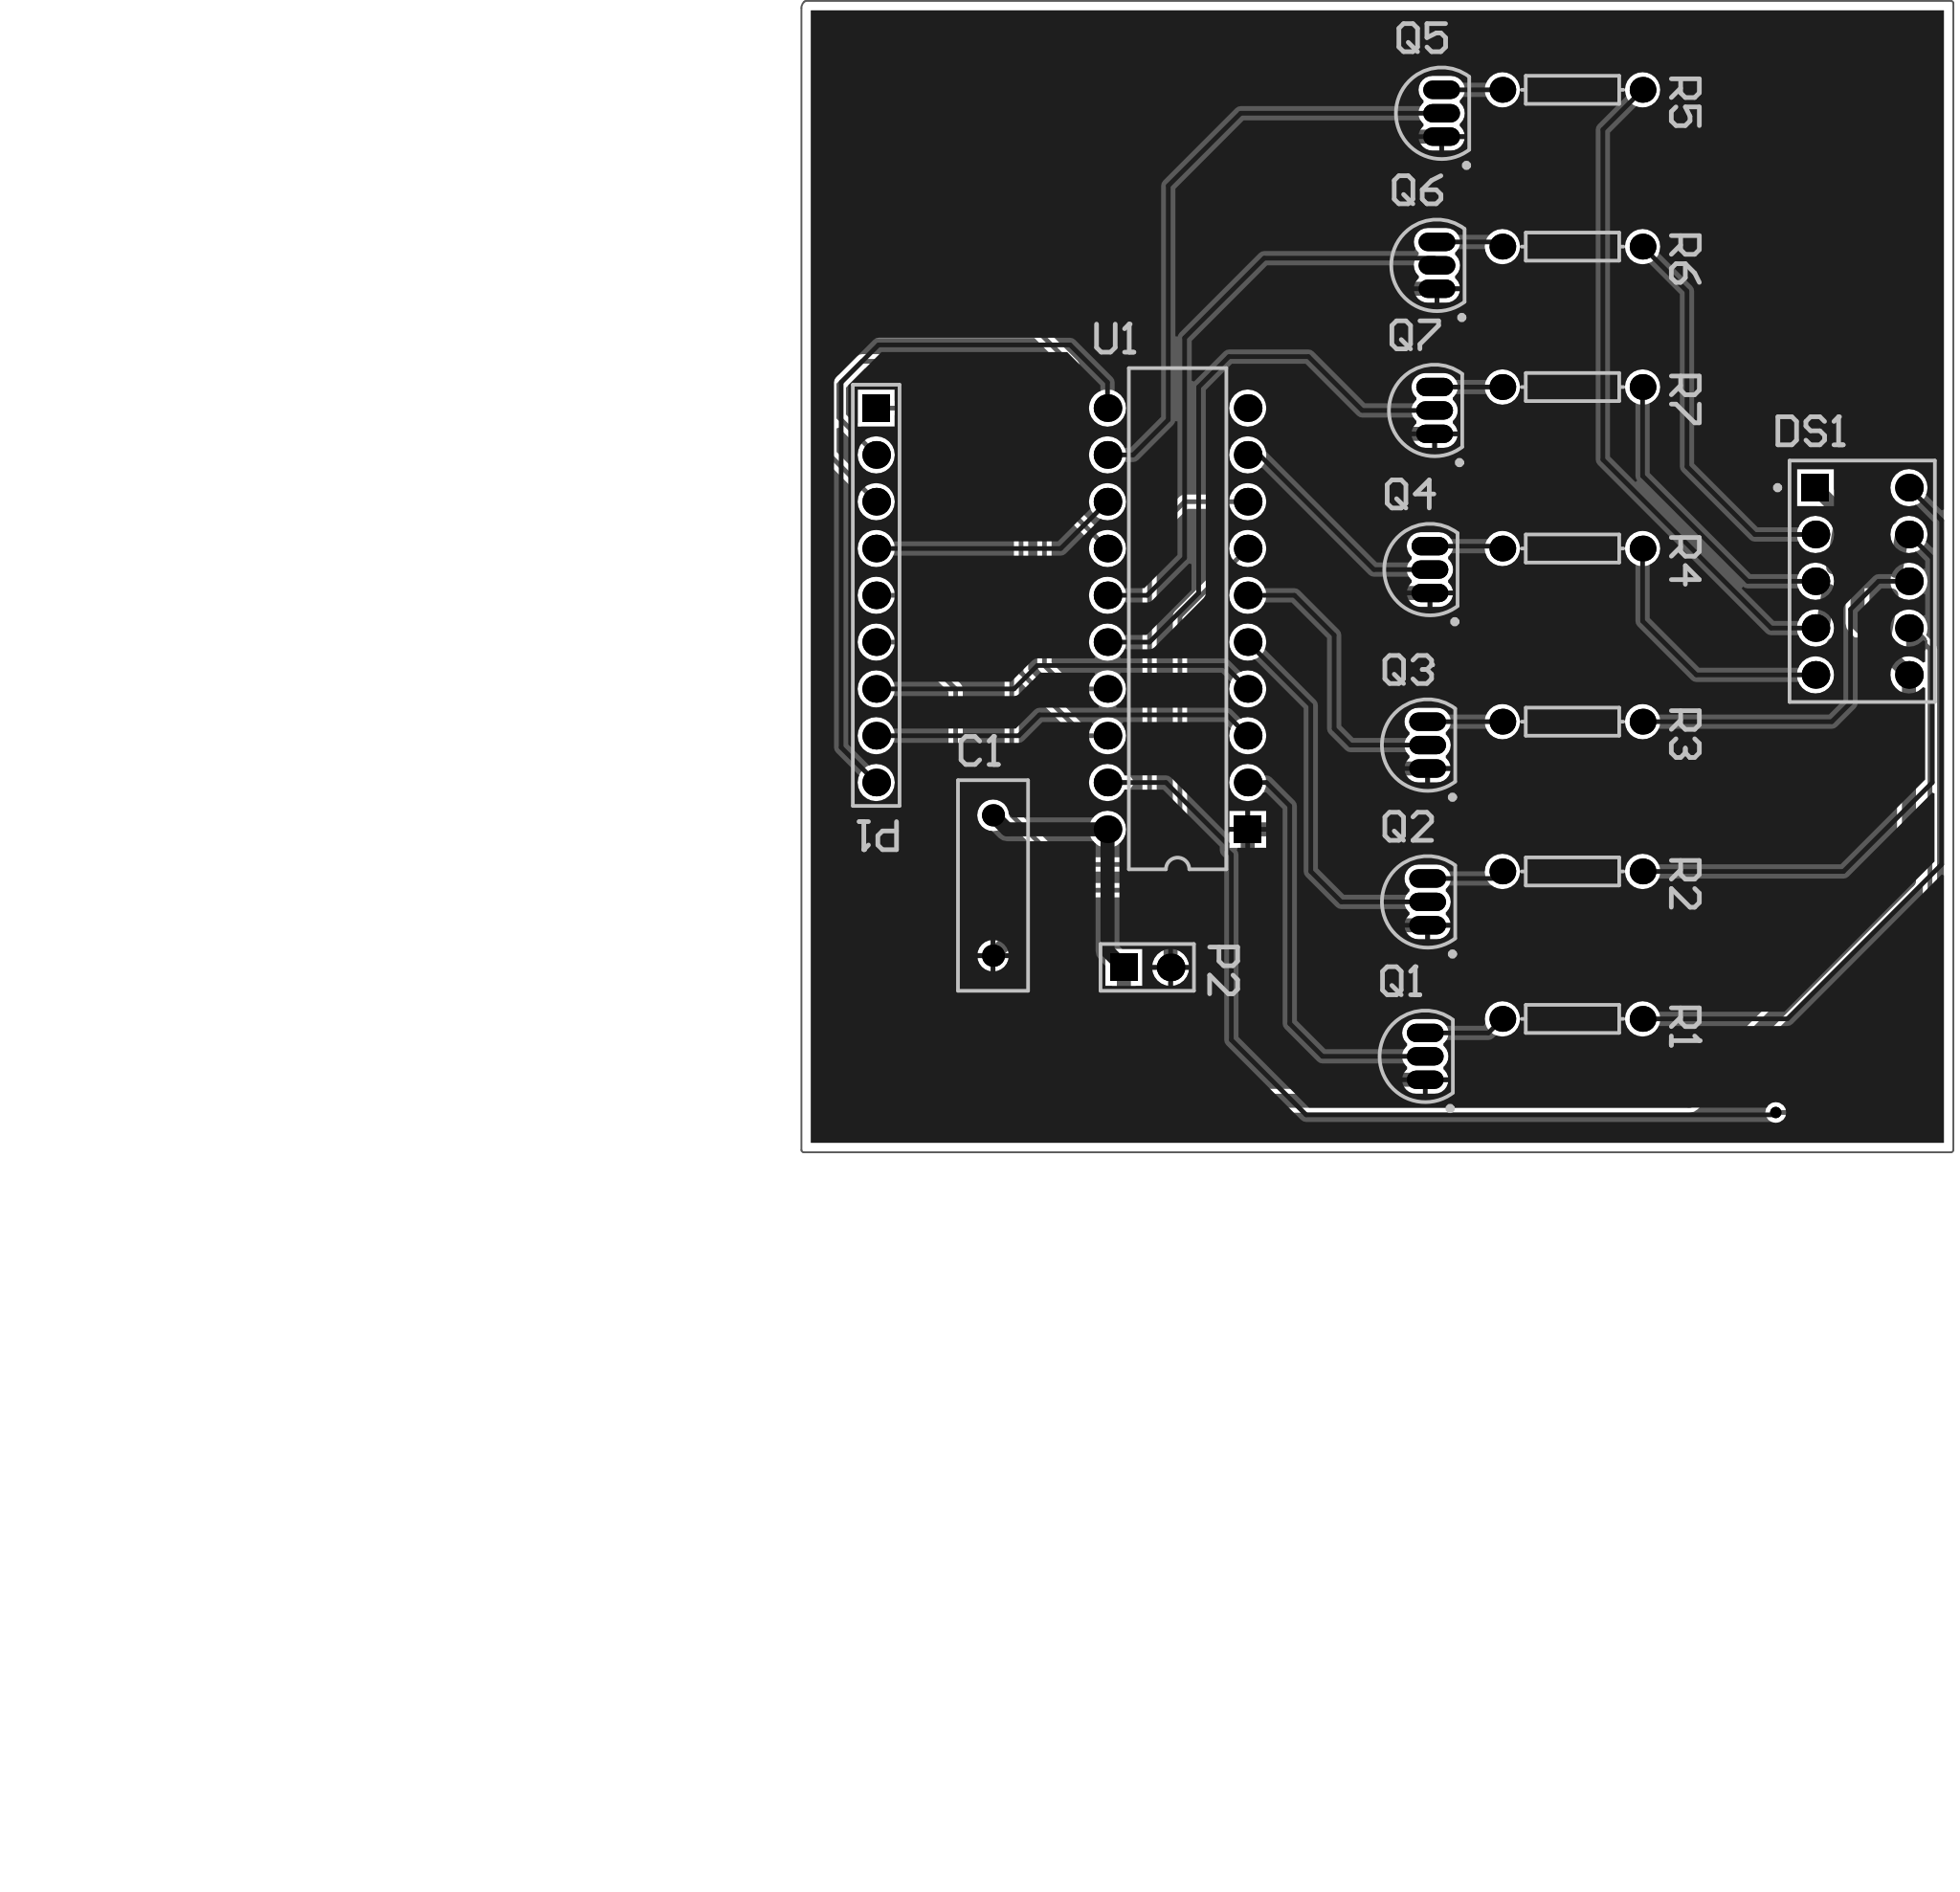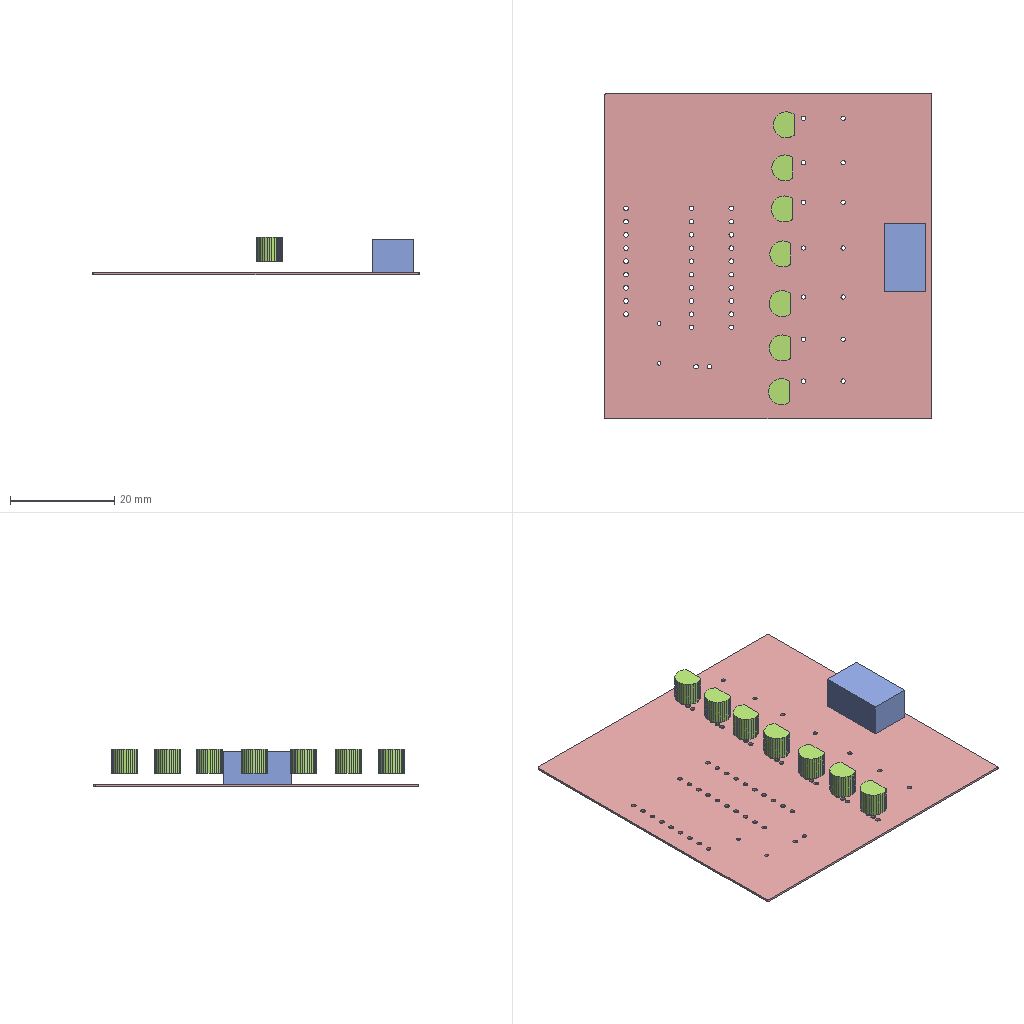Circuit board layout | Altium Designer | box 62.6 x 62.5 x 7.3 mm
Layer stack:
# Altium Designer layer stack of 2 (unit mm; dielectric type: 0 none, 1 core, 2 prepreg, 3 surface material)
index,name,kind,layer,copper_thickness_mm,dielectric_type,dielectric_thickness_mm,dielectric_material,dielectric_constant
0,Top Paste,other,,,,,,
1,Top Overlay,other,,,,,,
2,Top Solder,dielectric,,,3,0.0102,Solder Resist,3.5
3,Top Layer,copper,Top Layer,0.0356,,,,
4,Dielectric 1,dielectric,,,0,0.32,FR-4,4.8
5,Bottom Layer,copper,Bottom Layer,0.0356,,,,
6,Bottom Solder,dielectric,,,3,0.0102,Solder Resist,3.5
7,Bottom Overlay,other,,,,,,
8,Bottom Paste,other,,,,,,
# drill layer pairs: low layer,high layer
drill_pair,Top Layer,Bottom Layer
Part placement:
Designator,Comment,Layer,Footprint,Center-X(mm),Center-Y(mm),Rotation
C1,Value,TopLayer,RAD-0.3,53.975,54.356,90
DS1,Dpy Red-CA,TopLayer,A,101.219,70.866,360
P1,Header 9,TopLayer,HDR1X9,47.625,70.104,270
P2,Header 2,TopLayer,HDR1X2,62.357,49.911,360
Q1,2N222A,TopLayer,TO-92A,77.47,45.085,0
Q2,2N222A,TopLayer,TO-92A,77.597,53.467,0
Q3,2N222A,TopLayer,TO-92A,77.597,61.976,360
Q4,2N222A,TopLayer,TO-92A,77.724,71.501,0
Q5,2N222A,TopLayer,TO-92A,78.359,96.266,360
Q6,2N222A,TopLayer,TO-92A,78.105,88.011,0
Q7,2N222A,TopLayer,TO-92A,77.978,80.137,0
R1,Value,TopLayer,AXIAL-0.3,85.471,47.117,360
R2,Value,TopLayer,AXIAL-0.3,85.471,55.118,360
R3,Value,TopLayer,AXIAL-0.3,85.471,63.246,360
R4,Value,TopLayer,AXIAL-0.3,85.471,72.644,360
R5,Value,TopLayer,AXIAL-0.3,85.471,97.536,360
R6,Value,TopLayer,AXIAL-0.3,85.471,89.027,360
R7,Value,TopLayer,AXIAL-0.3,85.471,81.407,360
U1,SN74LS373N,TopLayer,738-03,64.008,68.834,90
Pad and via stacks:
# Altium Designer via and pad stacks of 2 (unit mm). Each distinct definition once, with the count of objects using it.
# via: kind,start_layer,end_layer,hole_mm,diameter_mm,mode(0 simple;1 top-mid-bottom;2 full stack),diameter_per_layer,count,example_net
# pad: kind,layer,hole_mm,hole_type(0 round;1 square;2 slot),plating,top_size,top_shape(1 round;2 rect;3 octagon;9 rounded rect),mid_size,bottom_size,mode,footprint,size_per_layer,count,example
pad,Multi-Layer,0.9,0,plated,2x1,1,2x1,2x1,0,TO-92A,,21,Q7.1
pad,Multi-Layer,0.85,0,plated,1.4x1.4,1,1.4x1.4,1.4x1.4,0,AXIAL-0.3,,14,R7.1
pad,Multi-Layer,0.9,0,plated,1.5x1.5,1,1.5x1.5,1.5x1.5,0,HDR1X2,,1,P2.2
pad,Multi-Layer,0.9,0,plated,1.5x1.5,2,1.5x1.5,1.5x1.5,0,HDR1X2,,1,P2.1
pad,Multi-Layer,0.9,0,plated,1.5x1.5,2,1.5x1.5,1.5x1.5,0,A,,1,DS1.1
pad,Multi-Layer,0.9,0,plated,1.5x1.5,1,1.5x1.5,1.5x1.5,0,A,,9,DS1.2
pad,Multi-Layer,0.9,0,plated,1.5x1.5,1,1.5x1.5,1.5x1.5,0,HDR1X9,,8,P1.2
pad,Multi-Layer,0.9,0,plated,1.5x1.5,2,1.5x1.5,1.5x1.5,0,HDR1X9,,1,P1.1
pad,Multi-Layer,0.9,0,plated,1.5x1.5,1,1.5x1.5,1.5x1.5,0,738-03,,19,U1.11
pad,Multi-Layer,0.9,0,plated,1.5x1.5,2,1.5x1.5,1.5x1.5,0,738-03,,1,U1.1
pad,Multi-Layer,0.7,0,plated,1.2x1.2,1,1.2x1.2,1.2x1.2,0,RAD-0.3,,2,C1.1
via,Top Layer,Bottom Layer,0.3048,0.6096,0,,1,NetDS1_7
Copper pours:
name,layer,net,type(0 solid;1 hatched;2 none)
D,Bottom Layer,GND,0
D,Top Layer,GND,0
Design rules, without the lines most boards share:
# Altium Designer design rules of 2 (exported by Altium Designer, unit mm)
# columns: name | kind | enabled | priority | scope1 | scope2 | descriptor | typed fields (field=value)
Clearance | 0 | enabled | 1 | All | All | Clearance Constraint (Gap=10mil) (All),(All) | gap=0.254
PlaneConnect | 6 | enabled | 1 | All | All | Power Plane Connect Rule(Relief Connect )(Expansion=20mil) (Conductor Width=10mil) (Air Gap=10mil) (Entries=4) (All) | relief_conductor_width=0.254 relief_entries=4 relief_expansion=0.508
PolygonConnect | 20 | enabled | 1 | All | All | Polygon Connect Rule(Relief Connect )(Conductor Width=10mil) (Relief Angle=90 Angle) (Entries=4) (Air Gap Width=10mil) (All),(All) | connect_style(0=relief,1=direct,2=none)=0 relief_conductor_width=0.254 relief_entries=4
Width | 2 | enabled | 1 | All | All | Width Constraint (Min=10mil) (Max=30mil) (Preferred=10mil) (All) |
RoutingVias | 11 | enabled | 1 | All | All | Routing Via (MinHoleWidth=28mil) (MaxHoleWidth=28mil) (PreferredHoleWidth=28mil) (MinWidth=50mil) (MaxWidth=50mil) (PreferedWidth=50mil) (All) | via_min_hole=0.7112 via_max_hole=0.7112 via_preferred_diameter=1.27 via_preferred_hole=0.7112
PasteMaskExpansion | 14 | enabled | 1 | All | All | Paste Mask Expansion (Expansion =0mil) (All) | expansion=0
SolderMaskExpansion | 13 | enabled | 1 | All | All | Solder Mask Expansion (Expansion =4mil) (All) | expansion=0.1016
DiffPairsRouting | 51 | enabled | 1 | All | All | Differential Pairs Uncoupled Length using the Gap Constraints (Min=10mil) (Max=10mil) (Prefered=10mil)  and Width Constraints (Min=15mil) (Max=15mil) (Prefered=15mil) (All) |
HoleToHoleClearance | 52 | enabled | 1 | All | All | Hole To Hole Clearance (Gap=10mil) (All),(All) | gap=0.254
MinimumSolderMaskSliver | 53 | enabled | 1 | All | All | Minimum Solder Mask Sliver (Gap=0mil) (All),(All) |
SilkToSolderMaskClearance | 54 | enabled | 1 | IsPad | All | Silk To Solder Mask (Clearance=0mil) (IsPad),(All) |
SilkToSilkClearance | 55 | enabled | 1 | All | All | Silk to Silk (Clearance=0mil) (All),(All) |
Classes set for this board:
# Altium Designer classes of 2 (member kind: 0 net, 1 component, 2 from-to, 3 pad, 4 layer, 5 differential pair, 6 design channel, 7 polygon, 8 structure, 9 xSignal)
# columns: class name | member kind | superclass | members
Sheet1 | 1 | no | C1; DS1; P1; P2; Q1; Q2; Q3; Q4; Q5; Q6; Q7; R1; R2; R3; R4; R5; R6; R7; U1;